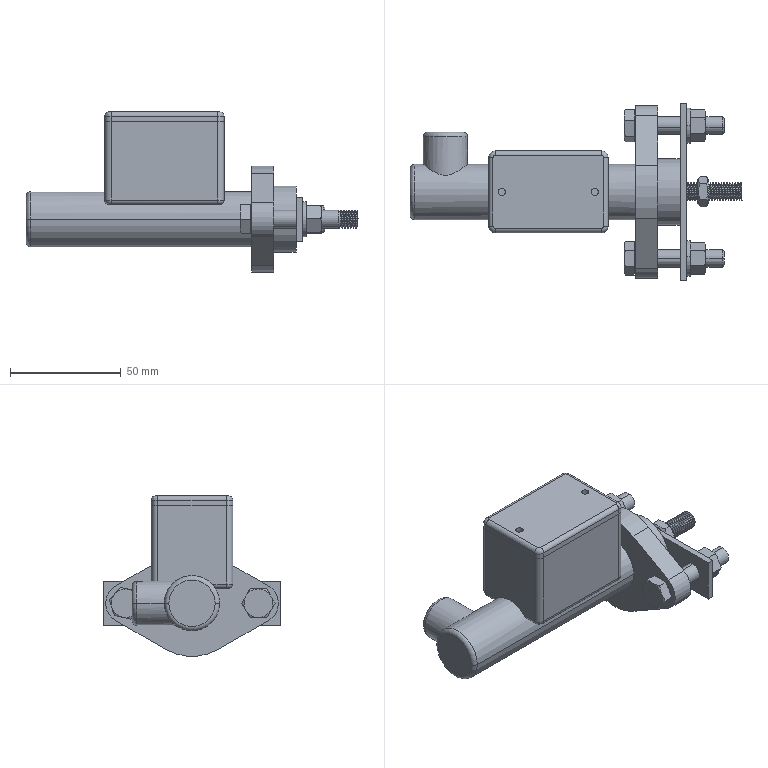Part | SolidWorks | 12 solids | 429 faces | box 150.004 x 80 x 72.5 mm | volume 111449 mm3 | cylinder 230 | plane 121 | cone 54 | torus 18 | spline 4 | sphere 2 | commonest cylinder face diameters 8 x69 6.75 x49 6 x12 7 x12 14 x12 4 x10